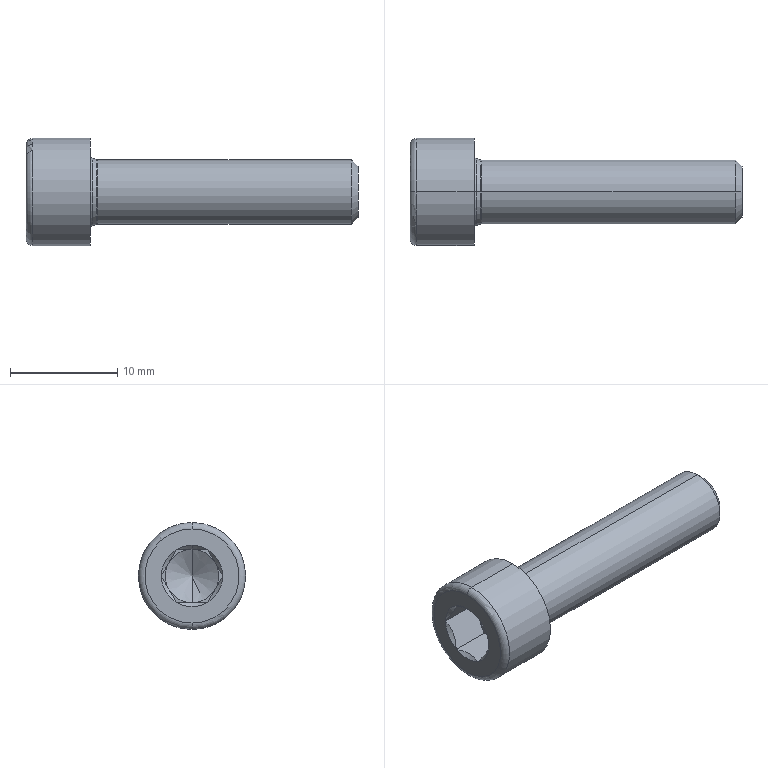Part | STEP file | 1 solid | 38 faces | box 31 x 10 x 10 mm | volume 1084 mm3 | plane 15 | cone 13 | torus 6 | cylinder 4 | commonest cylinder face diameters 6 x2 10 x2
STEP:
#1=CARTESIAN_POINT('',(-0.8566,0.,0.));
#2=VERTEX_POINT('',#1);
#3=CARTESIAN_POINT('',(-2.3,0.,2.5));
#4=VERTEX_POINT('',#3);
#5=CARTESIAN_POINT('',(-2.3,0.,2.5));
#6=DIRECTION('',(-0.5,0.,0.866));
#7=VECTOR('',#6,1000.);
#8=LINE('',#5,#7);
#9=EDGE_CURVE('',#2,#4,#8,.T.);
#10=ORIENTED_EDGE('',*,*,#9,.F.);
#11=CARTESIAN_POINT('',(-2.3,0.,-2.5));
#12=VERTEX_POINT('',#11);
#13=CARTESIAN_POINT('',(-2.3,0.,-2.5));
#14=DIRECTION('',(-0.5,0.,-0.866));
#15=VECTOR('',#14,1000.);
#16=LINE('',#13,#15);
#17=EDGE_CURVE('',#2,#12,#16,.T.);
#18=ORIENTED_EDGE('',*,*,#17,.T.);
#19=CARTESIAN_POINT('',(-2.3,-2.165,-1.25));
#20=VERTEX_POINT('',#19);
#21=CARTESIAN_POINT('',(-2.3,0.,0.));
#22=DIRECTION('',(-1.,0.,0.));
#23=DIRECTION('',(0.,0.,1.));
#24=AXIS2_PLACEMENT_3D('',#21,#22,#23);
#25=CIRCLE('',#24,2.5);
#26=EDGE_CURVE('',#12,#20,#25,.T.);
#27=ORIENTED_EDGE('',*,*,#26,.T.);
#28=CARTESIAN_POINT('',(-2.3,-2.165,1.25));
#29=VERTEX_POINT('',#28);
#30=CARTESIAN_POINT('',(-2.3,0.,0.));
#31=DIRECTION('',(-1.,0.,0.));
#32=DIRECTION('',(0.,0.,1.));
#33=AXIS2_PLACEMENT_3D('',#30,#31,#32);
#34=CIRCLE('',#33,2.5);
#35=EDGE_CURVE('',#20,#29,#34,.T.);
#36=ORIENTED_EDGE('',*,*,#35,.T.);
#37=CARTESIAN_POINT('',(-2.3,0.,0.));
#38=DIRECTION('',(-1.,0.,0.));
#39=DIRECTION('',(0.,0.,1.));
#40=AXIS2_PLACEMENT_3D('',#37,#38,#39);
#41=CIRCLE('',#40,2.5);
#42=EDGE_CURVE('',#29,#4,#41,.T.);
#43=ORIENTED_EDGE('',*,*,#42,.T.);
#44=EDGE_LOOP('',(#10,#18,#27,#36,#43));
#45=FACE_OUTER_BOUND('',#44,.T.);
#46=CARTESIAN_POINT('',(-2.3,0.,0.));
#47=DIRECTION('',(-1.,0.,0.));
#48=DIRECTION('',(0.,0.,1.));
#49=AXIS2_PLACEMENT_3D('',#46,#47,#48);
#50=CONICAL_SURFACE('',#49,2.5,1.047);
#51=ADVANCED_FACE('',(#45),#50,.F.);
#52=CARTESIAN_POINT('',(25.,0.,2.386));
#53=VERTEX_POINT('',#52);
#54=CARTESIAN_POINT('',(25.,0.,-2.386));
#55=VERTEX_POINT('',#54);
#56=CARTESIAN_POINT('',(25.,0.,0.));
#57=DIRECTION('',(-1.,0.,0.));
#58=DIRECTION('',(0.,0.,1.));
#59=AXIS2_PLACEMENT_3D('',#56,#57,#58);
#60=CIRCLE('',#59,2.386);
#61=EDGE_CURVE('',#53,#55,#60,.T.);
#62=ORIENTED_EDGE('',*,*,#61,.T.);
#63=CARTESIAN_POINT('',(24.386,0.,-3.));
#64=VERTEX_POINT('',#63);
#65=CARTESIAN_POINT('',(25.,0.,-2.386));
#66=DIRECTION('',(-0.7071,0.,-0.7071));
#67=VECTOR('',#66,1000.);
#68=LINE('',#65,#67);
#69=EDGE_CURVE('',#55,#64,#68,.T.);
#70=ORIENTED_EDGE('',*,*,#69,.T.);
#71=CARTESIAN_POINT('',(24.386,0.,3.));
#72=VERTEX_POINT('',#71);
#73=CARTESIAN_POINT('',(24.386,0.,0.));
#74=DIRECTION('',(-1.,0.,0.));
#75=DIRECTION('',(0.,0.,1.));
#76=AXIS2_PLACEMENT_3D('',#73,#74,#75);
#77=CIRCLE('',#76,3.);
#78=EDGE_CURVE('',#72,#64,#77,.T.);
#79=ORIENTED_EDGE('',*,*,#78,.F.);
#80=CARTESIAN_POINT('',(25.,0.,2.386));
#81=DIRECTION('',(-0.7071,0.,0.7071));
#82=VECTOR('',#81,1000.);
#83=LINE('',#80,#82);
#84=EDGE_CURVE('',#53,#72,#83,.T.);
#85=ORIENTED_EDGE('',*,*,#84,.F.);
#86=EDGE_LOOP('',(#62,#70,#79,#85));
#87=FACE_OUTER_BOUND('',#86,.T.);
#88=CARTESIAN_POINT('',(25.,0.,0.));
#89=DIRECTION('',(-1.,0.,0.));
#90=DIRECTION('',(0.,0.,1.));
#91=AXIS2_PLACEMENT_3D('',#88,#89,#90);
#92=CONICAL_SURFACE('',#91,2.386,0.7854);
#93=ADVANCED_FACE('',(#87),#92,.T.);
#94=ORIENTED_EDGE('',*,*,#78,.T.);
#95=CARTESIAN_POINT('',(0.68,0.,-3.));
#96=VERTEX_POINT('',#95);
#97=CARTESIAN_POINT('',(28.,0.,-3.));
#98=DIRECTION('',(-1.,0.,0.));
#99=VECTOR('',#98,1000.);
#100=LINE('',#97,#99);
#101=EDGE_CURVE('',#64,#96,#100,.T.);
#102=ORIENTED_EDGE('',*,*,#101,.T.);
#103=CARTESIAN_POINT('',(0.68,0.,3.));
#104=VERTEX_POINT('',#103);
#105=CARTESIAN_POINT('',(0.68,0.,0.));
#106=DIRECTION('',(-1.,0.,0.));
#107=DIRECTION('',(0.,0.,1.));
#108=AXIS2_PLACEMENT_3D('',#105,#106,#107);
#109=CIRCLE('',#108,3.);
#110=EDGE_CURVE('',#104,#96,#109,.T.);
#111=ORIENTED_EDGE('',*,*,#110,.F.);
#112=CARTESIAN_POINT('',(28.,0.,3.));
#113=DIRECTION('',(-1.,0.,0.));
#114=VECTOR('',#113,1000.);
#115=LINE('',#112,#114);
#116=EDGE_CURVE('',#72,#104,#115,.T.);
#117=ORIENTED_EDGE('',*,*,#116,.F.);
#118=EDGE_LOOP('',(#94,#102,#111,#117));
#119=FACE_OUTER_BOUND('',#118,.T.);
#120=CARTESIAN_POINT('',(28.,0.,0.));
#121=DIRECTION('',(-1.,0.,0.));
#122=DIRECTION('',(0.,0.,1.));
#123=AXIS2_PLACEMENT_3D('',#120,#121,#122);
#124=CYLINDRICAL_SURFACE('',#123,3.);
#125=ADVANCED_FACE('',(#119),#124,.T.);
#126=CARTESIAN_POINT('',(0.5977,0.,-3.014));
#127=VERTEX_POINT('',#126);
#128=CARTESIAN_POINT('',(0.5977,0.,3.014));
#129=VERTEX_POINT('',#128);
#130=CARTESIAN_POINT('',(0.5977,0.,0.));
#131=DIRECTION('',(-1.,0.,0.));
#132=DIRECTION('',(0.,0.,1.));
#133=AXIS2_PLACEMENT_3D('',#130,#131,#132);
#134=CIRCLE('',#133,3.014);
#135=EDGE_CURVE('',#127,#129,#134,.T.);
#136=ORIENTED_EDGE('',*,*,#135,.F.);
#137=CARTESIAN_POINT('',(0.68,0.,-3.25));
#138=DIRECTION('',(0.,1.,0.));
#139=DIRECTION('',(0.,0.,1.));
#140=AXIS2_PLACEMENT_3D('',#137,#138,#139);
#141=CIRCLE('',#140,0.25);
#142=EDGE_CURVE('',#127,#96,#141,.T.);
#143=ORIENTED_EDGE('',*,*,#142,.T.);
#144=CARTESIAN_POINT('',(0.68,0.,0.));
#145=DIRECTION('',(-1.,0.,0.));
#146=DIRECTION('',(0.,0.,1.));
#147=AXIS2_PLACEMENT_3D('',#144,#145,#146);
#148=CIRCLE('',#147,3.);
#149=EDGE_CURVE('',#96,#104,#148,.T.);
#150=ORIENTED_EDGE('',*,*,#149,.T.);
#151=CARTESIAN_POINT('',(0.68,0.,3.25));
#152=DIRECTION('',(0.,-1.,0.));
#153=DIRECTION('',(0.,0.,-1.));
#154=AXIS2_PLACEMENT_3D('',#151,#152,#153);
#155=CIRCLE('',#154,0.25);
#156=EDGE_CURVE('',#129,#104,#155,.T.);
#157=ORIENTED_EDGE('',*,*,#156,.F.);
#158=EDGE_LOOP('',(#136,#143,#150,#157));
#159=FACE_OUTER_BOUND('',#158,.T.);
#160=CARTESIAN_POINT('',(0.68,0.,0.));
#161=DIRECTION('',(-1.,0.,0.));
#162=DIRECTION('',(0.,0.,1.));
#163=AXIS2_PLACEMENT_3D('',#160,#161,#162);
#164=TOROIDAL_SURFACE('',#163,3.25,0.25);
#165=ADVANCED_FACE('',(#159),#164,.F.);
#166=CARTESIAN_POINT('',(0.5977,0.,0.));
#167=DIRECTION('',(-1.,0.,0.));
#168=DIRECTION('',(0.,0.,1.));
#169=AXIS2_PLACEMENT_3D('',#166,#167,#168);
#170=CIRCLE('',#169,3.014);
#171=EDGE_CURVE('',#129,#127,#170,.T.);
#172=ORIENTED_EDGE('',*,*,#171,.T.);
#173=CARTESIAN_POINT('',(0.1677,0.,-3.164));
#174=VERTEX_POINT('',#173);
#175=CARTESIAN_POINT('',(0.5977,0.,-3.014));
#176=DIRECTION('',(-0.9442,0.,-0.3294));
#177=VECTOR('',#176,1000.);
#178=LINE('',#175,#177);
#179=EDGE_CURVE('',#127,#174,#178,.T.);
#180=ORIENTED_EDGE('',*,*,#179,.T.);
#181=CARTESIAN_POINT('',(0.1677,0.,3.164));
#182=VERTEX_POINT('',#181);
#183=CARTESIAN_POINT('',(0.1677,0.,0.));
#184=DIRECTION('',(-1.,0.,0.));
#185=DIRECTION('',(0.,0.,1.));
#186=AXIS2_PLACEMENT_3D('',#183,#184,#185);
#187=CIRCLE('',#186,3.164);
#188=EDGE_CURVE('',#182,#174,#187,.T.);
#189=ORIENTED_EDGE('',*,*,#188,.F.);
#190=CARTESIAN_POINT('',(0.5977,0.,3.014));
#191=DIRECTION('',(-0.9442,0.,0.3294));
#192=VECTOR('',#191,1000.);
#193=LINE('',#190,#192);
#194=EDGE_CURVE('',#129,#182,#193,.T.);
#195=ORIENTED_EDGE('',*,*,#194,.F.);
#196=EDGE_LOOP('',(#172,#180,#189,#195));
#197=FACE_OUTER_BOUND('',#196,.T.);
#198=CARTESIAN_POINT('',(0.5977,0.,0.));
#199=DIRECTION('',(-1.,0.,0.));
#200=DIRECTION('',(0.,0.,1.));
#201=AXIS2_PLACEMENT_3D('',#198,#199,#200);
#202=CONICAL_SURFACE('',#201,3.014,0.3356);
#203=ADVANCED_FACE('',(#197),#202,.T.);
#204=CARTESIAN_POINT('',(0.,0.,-3.4));
#205=VERTEX_POINT('',#204);
#206=CARTESIAN_POINT('',(0.,0.,3.4));
#207=VERTEX_POINT('',#206);
#208=CARTESIAN_POINT('',(0.,0.,0.));
#209=DIRECTION('',(-1.,0.,0.));
#210=DIRECTION('',(0.,0.,1.));
#211=AXIS2_PLACEMENT_3D('',#208,#209,#210);
#212=CIRCLE('',#211,3.4);
#213=EDGE_CURVE('',#205,#207,#212,.T.);
#214=ORIENTED_EDGE('',*,*,#213,.F.);
#215=CARTESIAN_POINT('',(0.25,0.,-3.4));
#216=DIRECTION('',(0.,1.,0.));
#217=DIRECTION('',(0.,0.,1.));
#218=AXIS2_PLACEMENT_3D('',#215,#216,#217);
#219=CIRCLE('',#218,0.25);
#220=EDGE_CURVE('',#205,#174,#219,.T.);
#221=ORIENTED_EDGE('',*,*,#220,.T.);
#222=CARTESIAN_POINT('',(0.1677,0.,0.));
#223=DIRECTION('',(-1.,0.,0.));
#224=DIRECTION('',(0.,0.,1.));
#225=AXIS2_PLACEMENT_3D('',#222,#223,#224);
#226=CIRCLE('',#225,3.164);
#227=EDGE_CURVE('',#174,#182,#226,.T.);
#228=ORIENTED_EDGE('',*,*,#227,.T.);
#229=CARTESIAN_POINT('',(0.25,0.,3.4));
#230=DIRECTION('',(0.,-1.,0.));
#231=DIRECTION('',(0.,0.,-1.));
#232=AXIS2_PLACEMENT_3D('',#229,#230,#231);
#233=CIRCLE('',#232,0.25);
#234=EDGE_CURVE('',#207,#182,#233,.T.);
#235=ORIENTED_EDGE('',*,*,#234,.F.);
#236=EDGE_LOOP('',(#214,#221,#228,#235));
#237=FACE_OUTER_BOUND('',#236,.T.);
#238=CARTESIAN_POINT('',(0.25,0.,0.));
#239=DIRECTION('',(-1.,0.,0.));
#240=DIRECTION('',(0.,0.,1.));
#241=AXIS2_PLACEMENT_3D('',#238,#239,#240);
#242=TOROIDAL_SURFACE('',#241,3.4,0.25);
#243=ADVANCED_FACE('',(#237),#242,.F.);
#244=CARTESIAN_POINT('',(0.,0.,5.));
#245=VERTEX_POINT('',#244);
#246=CARTESIAN_POINT('',(0.,0.,-5.));
#247=VERTEX_POINT('',#246);
#248=CARTESIAN_POINT('',(0.,0.,0.));
#249=DIRECTION('',(-1.,0.,0.));
#250=DIRECTION('',(0.,0.,1.));
#251=AXIS2_PLACEMENT_3D('',#248,#249,#250);
#252=CIRCLE('',#251,5.);
#253=EDGE_CURVE('',#245,#247,#252,.T.);
#254=ORIENTED_EDGE('',*,*,#253,.T.);
#255=CARTESIAN_POINT('',(-5.4,0.,-5.));
#256=VERTEX_POINT('',#255);
#257=CARTESIAN_POINT('',(28.,0.,-5.));
#258=DIRECTION('',(-1.,0.,0.));
#259=VECTOR('',#258,1000.);
#260=LINE('',#257,#259);
#261=EDGE_CURVE('',#247,#256,#260,.T.);
#262=ORIENTED_EDGE('',*,*,#261,.T.);
#263=CARTESIAN_POINT('',(-5.4,0.,5.));
#264=VERTEX_POINT('',#263);
#265=CARTESIAN_POINT('',(-5.4,0.,0.));
#266=DIRECTION('',(-1.,0.,0.));
#267=DIRECTION('',(0.,0.,1.));
#268=AXIS2_PLACEMENT_3D('',#265,#266,#267);
#269=CIRCLE('',#268,5.);
#270=EDGE_CURVE('',#264,#256,#269,.T.);
#271=ORIENTED_EDGE('',*,*,#270,.F.);
#272=CARTESIAN_POINT('',(28.,0.,5.));
#273=DIRECTION('',(-1.,0.,0.));
#274=VECTOR('',#273,1000.);
#275=LINE('',#272,#274);
#276=EDGE_CURVE('',#245,#264,#275,.T.);
#277=ORIENTED_EDGE('',*,*,#276,.F.);
#278=EDGE_LOOP('',(#254,#262,#271,#277));
#279=FACE_OUTER_BOUND('',#278,.T.);
#280=CARTESIAN_POINT('',(28.,0.,0.));
#281=DIRECTION('',(-1.,0.,0.));
#282=DIRECTION('',(0.,0.,1.));
#283=AXIS2_PLACEMENT_3D('',#280,#281,#282);
#284=CYLINDRICAL_SURFACE('',#283,5.);
#285=ADVANCED_FACE('',(#279),#284,.T.);
#286=ORIENTED_EDGE('',*,*,#270,.T.);
#287=CARTESIAN_POINT('',(-6.,0.,-4.4));
#288=VERTEX_POINT('',#287);
#289=CARTESIAN_POINT('',(-5.4,0.,-4.4));
#290=DIRECTION('',(0.,1.,0.));
#291=DIRECTION('',(0.,0.,1.));
#292=AXIS2_PLACEMENT_3D('',#289,#290,#291);
#293=CIRCLE('',#292,0.6);
#294=EDGE_CURVE('',#256,#288,#293,.T.);
#295=ORIENTED_EDGE('',*,*,#294,.T.);
#296=CARTESIAN_POINT('',(-6.,0.,4.4));
#297=VERTEX_POINT('',#296);
#298=CARTESIAN_POINT('',(-6.,0.,0.));
#299=DIRECTION('',(-1.,0.,0.));
#300=DIRECTION('',(0.,0.,1.));
#301=AXIS2_PLACEMENT_3D('',#298,#299,#300);
#302=CIRCLE('',#301,4.4);
#303=EDGE_CURVE('',#297,#288,#302,.T.);
#304=ORIENTED_EDGE('',*,*,#303,.F.);
#305=CARTESIAN_POINT('',(-5.4,0.,4.4));
#306=DIRECTION('',(0.,-1.,0.));
#307=DIRECTION('',(0.,0.,-1.));
#308=AXIS2_PLACEMENT_3D('',#305,#306,#307);
#309=CIRCLE('',#308,0.6);
#310=EDGE_CURVE('',#264,#297,#309,.T.);
#311=ORIENTED_EDGE('',*,*,#310,.F.);
#312=EDGE_LOOP('',(#286,#295,#304,#311));
#313=FACE_OUTER_BOUND('',#312,.T.);
#314=CARTESIAN_POINT('',(-5.4,0.,0.));
#315=DIRECTION('',(-1.,0.,0.));
#316=DIRECTION('',(0.,0.,1.));
#317=AXIS2_PLACEMENT_3D('',#314,#315,#316);
#318=TOROIDAL_SURFACE('',#317,4.4,0.6);
#319=ADVANCED_FACE('',(#313),#318,.T.);
#320=CARTESIAN_POINT('',(-6.,1.389,2.5));
#321=VERTEX_POINT('',#320);
#322=CARTESIAN_POINT('',(-5.64,0.,2.5));
#323=VERTEX_POINT('',#322);
#324=CARTESIAN_POINT('',(-6.,1.389,2.5));
#325=CARTESIAN_POINT('',(-5.895,1.173,2.5));
#326=CARTESIAN_POINT('',(-5.804,0.9463,2.5));
#327=CARTESIAN_POINT('',(-5.676,0.481,2.5));
#328=CARTESIAN_POINT('',(-5.64,0.2436,2.5));
#329=CARTESIAN_POINT('',(-5.64,0.,2.5));
#330=B_SPLINE_CURVE_WITH_KNOTS('',3,(#324,#325,#326,#327,#328,#329),.UNSPECIFIED.,.F.,.F.,(4,2,4),(0.001597,0.002315,0.003033),.UNSPECIFIED.);
#331=EDGE_CURVE('',#321,#323,#330,.T.);
#332=ORIENTED_EDGE('',*,*,#331,.T.);
#333=CARTESIAN_POINT('',(-6.,0.,2.86));
#334=VERTEX_POINT('',#333);
#335=CARTESIAN_POINT('',(-6.,0.,2.86));
#336=DIRECTION('',(-0.7071,0.,0.7071));
#337=VECTOR('',#336,1000.);
#338=LINE('',#335,#337);
#339=EDGE_CURVE('',#323,#334,#338,.T.);
#340=ORIENTED_EDGE('',*,*,#339,.T.);
#341=CARTESIAN_POINT('',(-6.,0.,0.));
#342=DIRECTION('',(-1.,0.,0.));
#343=DIRECTION('',(0.,0.,1.));
#344=AXIS2_PLACEMENT_3D('',#341,#342,#343);
#345=CIRCLE('',#344,2.86);
#346=EDGE_CURVE('',#334,#321,#345,.T.);
#347=ORIENTED_EDGE('',*,*,#346,.T.);
#348=EDGE_LOOP('',(#332,#340,#347));
#349=FACE_OUTER_BOUND('',#348,.T.);
#350=CARTESIAN_POINT('',(-6.,0.,0.));
#351=DIRECTION('',(-1.,0.,0.));
#352=DIRECTION('',(0.,0.,1.));
#353=AXIS2_PLACEMENT_3D('',#350,#351,#352);
#354=CONICAL_SURFACE('',#353,2.86,0.7854);
#355=ADVANCED_FACE('',(#349),#354,.F.);
#356=CARTESIAN_POINT('',(-6.,1.471,2.453));
#357=VERTEX_POINT('',#356);
#358=CARTESIAN_POINT('',(-6.,2.86,0.047));
#359=VERTEX_POINT('',#358);
#360=CARTESIAN_POINT('',(-6.,0.,0.));
#361=DIRECTION('',(-1.,0.,0.));
#362=DIRECTION('',(0.,0.,1.));
#363=AXIS2_PLACEMENT_3D('',#360,#361,#362);
#364=CIRCLE('',#363,2.86);
#365=EDGE_CURVE('',#357,#359,#364,.T.);
#366=ORIENTED_EDGE('',*,*,#365,.T.);
#367=CARTESIAN_POINT('',(-6.,2.86,0.047));
#368=CARTESIAN_POINT('',(-5.894,2.751,0.2356));
#369=CARTESIAN_POINT('',(-5.805,2.639,0.4284));
#370=CARTESIAN_POINT('',(-5.709,2.467,0.7273));
#371=CARTESIAN_POINT('',(-5.684,2.408,0.8286));
#372=CARTESIAN_POINT('',(-5.65,2.289,1.035));
#373=CARTESIAN_POINT('',(-5.64,2.228,1.141));
#374=CARTESIAN_POINT('',(-5.64,2.046,1.456));
#375=CARTESIAN_POINT('',(-5.675,1.927,1.661));
#376=CARTESIAN_POINT('',(-5.803,1.693,2.068));
#377=CARTESIAN_POINT('',(-5.894,1.58,2.263));
#378=CARTESIAN_POINT('',(-6.,1.471,2.453));
#379=B_SPLINE_CURVE_WITH_KNOTS('',3,(#367,#368,#369,#370,#371,#372,#373,#374,#375,#376,#377,#378),.UNSPECIFIED.,.F.,.F.,(4,2,2,2,2,4),(0.000000451,0.0007165,0.001075,0.001433,0.002149,0.002865),.UNSPECIFIED.);
#380=EDGE_CURVE('',#359,#357,#379,.T.);
#381=ORIENTED_EDGE('',*,*,#380,.T.);
#382=EDGE_LOOP('',(#366,#381));
#383=FACE_OUTER_BOUND('',#382,.T.);
#384=CARTESIAN_POINT('',(-6.,0.,0.));
#385=DIRECTION('',(-1.,0.,0.));
#386=DIRECTION('',(0.,0.,1.));
#387=AXIS2_PLACEMENT_3D('',#384,#385,#386);
#388=CONICAL_SURFACE('',#387,2.86,0.7854);
#389=ADVANCED_FACE('',(#383),#388,.F.);
#390=CARTESIAN_POINT('',(-6.,2.86,-0.047));
#391=VERTEX_POINT('',#390);
#392=CARTESIAN_POINT('',(-6.,1.471,-2.453));
#393=VERTEX_POINT('',#392);
#394=CARTESIAN_POINT('',(-6.,0.,0.));
#395=DIRECTION('',(-1.,0.,0.));
#396=DIRECTION('',(0.,0.,1.));
#397=AXIS2_PLACEMENT_3D('',#394,#395,#396);
#398=CIRCLE('',#397,2.86);
#399=EDGE_CURVE('',#391,#393,#398,.T.);
#400=ORIENTED_EDGE('',*,*,#399,.T.);
#401=CARTESIAN_POINT('',(-6.,1.471,-2.453));
#402=CARTESIAN_POINT('',(-5.894,1.579,-2.264));
#403=CARTESIAN_POINT('',(-5.805,1.691,-2.072));
#404=CARTESIAN_POINT('',(-5.709,1.863,-1.773));
#405=CARTESIAN_POINT('',(-5.684,1.922,-1.671));
#406=CARTESIAN_POINT('',(-5.65,2.041,-1.465));
#407=CARTESIAN_POINT('',(-5.64,2.102,-1.359));
#408=CARTESIAN_POINT('',(-5.64,2.284,-1.044));
#409=CARTESIAN_POINT('',(-5.675,2.403,-0.8385));
#410=CARTESIAN_POINT('',(-5.803,2.637,-0.4324));
#411=CARTESIAN_POINT('',(-5.894,2.75,-0.2366));
#412=CARTESIAN_POINT('',(-6.,2.86,-0.047));
#413=B_SPLINE_CURVE_WITH_KNOTS('',3,(#401,#402,#403,#404,#405,#406,#407,#408,#409,#410,#411,#412),.UNSPECIFIED.,.F.,.F.,(4,2,2,2,2,4),(0.000000451,0.0007165,0.001075,0.001433,0.002149,0.002865),.UNSPECIFIED.);
#414=EDGE_CURVE('',#393,#391,#413,.T.);
#415=ORIENTED_EDGE('',*,*,#414,.T.);
#416=EDGE_LOOP('',(#400,#415));
#417=FACE_OUTER_BOUND('',#416,.T.);
#418=CARTESIAN_POINT('',(-6.,0.,0.));
#419=DIRECTION('',(-1.,0.,0.));
#420=DIRECTION('',(0.,0.,1.));
#421=AXIS2_PLACEMENT_3D('',#418,#419,#420);
#422=CONICAL_SURFACE('',#421,2.86,0.7854);
#423=ADVANCED_FACE('',(#417),#422,.F.);
#424=CARTESIAN_POINT('',(-6.,1.389,-2.5));
#425=VERTEX_POINT('',#424);
#426=CARTESIAN_POINT('',(-6.,-1.389,-2.5));
#427=VERTEX_POINT('',#426);
#428=CARTESIAN_POINT('',(-6.,0.,0.));
#429=DIRECTION('',(-1.,0.,0.));
#430=DIRECTION('',(0.,0.,1.));
#431=AXIS2_PLACEMENT_3D('',#428,#429,#430);
#432=CIRCLE('',#431,2.86);
#433=EDGE_CURVE('',#425,#427,#432,.T.);
#434=ORIENTED_EDGE('',*,*,#433,.T.);
#435=CARTESIAN_POINT('',(-6.,-1.389,-2.5));
#436=CARTESIAN_POINT('',(-5.895,-1.173,-2.5));
#437=CARTESIAN_POINT('',(-5.804,-0.9455,-2.5));
#438=CARTESIAN_POINT('',(-5.676,-0.482,-2.5));
#439=CARTESIAN_POINT('',(-5.64,-0.2429,-2.5));
#440=CARTESIAN_POINT('',(-5.64,0.2441,-2.5));
#441=CARTESIAN_POINT('',(-5.676,0.4814,-2.5));
#442=CARTESIAN_POINT('',(-5.804,0.9465,-2.5));
#443=CARTESIAN_POINT('',(-5.895,1.173,-2.5));
#444=CARTESIAN_POINT('',(-6.,1.389,-2.5));
#445=B_SPLINE_CURVE_WITH_KNOTS('',3,(#435,#436,#437,#438,#439,#440,#441,#442,#443,#444),.UNSPECIFIED.,.F.,.F.,(4,2,2,2,4),(0.001921,0.002639,0.003357,0.004076,0.004794),.UNSPECIFIED.);
#446=EDGE_CURVE('',#427,#425,#445,.T.);
#447=ORIENTED_EDGE('',*,*,#446,.T.);
#448=EDGE_LOOP('',(#434,#447));
#449=FACE_OUTER_BOUND('',#448,.T.);
#450=CARTESIAN_POINT('',(-6.,0.,0.));
#451=DIRECTION('',(-1.,0.,0.));
#452=DIRECTION('',(0.,0.,1.));
#453=AXIS2_PLACEMENT_3D('',#450,#451,#452);
#454=CONICAL_SURFACE('',#453,2.86,0.7854);
#455=ADVANCED_FACE('',(#449),#454,.F.);
#456=CARTESIAN_POINT('',(-6.,-1.471,-2.453));
#457=VERTEX_POINT('',#456);
#458=CARTESIAN_POINT('',(-6.,-2.86,-0.047));
#459=VERTEX_POINT('',#458);
#460=CARTESIAN_POINT('',(-6.,0.,0.));
#461=DIRECTION('',(-1.,0.,0.));
#462=DIRECTION('',(0.,0.,1.));
#463=AXIS2_PLACEMENT_3D('',#460,#461,#462);
#464=CIRCLE('',#463,2.86);
#465=EDGE_CURVE('',#457,#459,#464,.T.);
#466=ORIENTED_EDGE('',*,*,#465,.T.);
#467=CARTESIAN_POINT('',(-6.,-2.86,-0.047));
#468=CARTESIAN_POINT('',(-5.894,-2.751,-0.2356));
#469=CARTESIAN_POINT('',(-5.805,-2.639,-0.4284));
#470=CARTESIAN_POINT('',(-5.709,-2.467,-0.7273));
#471=CARTESIAN_POINT('',(-5.684,-2.408,-0.8286));
#472=CARTESIAN_POINT('',(-5.65,-2.289,-1.035));
#473=CARTESIAN_POINT('',(-5.64,-2.228,-1.141));
#474=CARTESIAN_POINT('',(-5.64,-2.046,-1.456));
#475=CARTESIAN_POINT('',(-5.675,-1.927,-1.661));
#476=CARTESIAN_POINT('',(-5.803,-1.693,-2.068));
#477=CARTESIAN_POINT('',(-5.894,-1.58,-2.263));
#478=CARTESIAN_POINT('',(-6.,-1.471,-2.453));
#479=B_SPLINE_CURVE_WITH_KNOTS('',3,(#467,#468,#469,#470,#471,#472,#473,#474,#475,#476,#477,#478),.UNSPECIFIED.,.F.,.F.,(4,2,2,2,2,4),(0.000000451,0.0007165,0.001075,0.001433,0.002149,0.002865),.UNSPECIFIED.);
#480=EDGE_CURVE('',#459,#457,#479,.T.);
#481=ORIENTED_EDGE('',*,*,#480,.T.);
#482=EDGE_LOOP('',(#466,#481));
#483=FACE_OUTER_BOUND('',#482,.T.);
#484=CARTESIAN_POINT('',(-6.,0.,0.));
#485=DIRECTION('',(-1.,0.,0.));
#486=DIRECTION('',(0.,0.,1.));
#487=AXIS2_PLACEMENT_3D('',#484,#485,#486);
#488=CONICAL_SURFACE('',#487,2.86,0.7854);
#489=ADVANCED_FACE('',(#483),#488,.F.);
#490=CARTESIAN_POINT('',(-6.,-2.86,0.047));
#491=VERTEX_POINT('',#490);
#492=CARTESIAN_POINT('',(-6.,-1.471,2.453));
#493=VERTEX_POINT('',#492);
#494=CARTESIAN_POINT('',(-6.,0.,0.));
#495=DIRECTION('',(-1.,0.,0.));
#496=DIRECTION('',(0.,0.,1.));
#497=AXIS2_PLACEMENT_3D('',#494,#495,#496);
#498=CIRCLE('',#497,2.86);
#499=EDGE_CURVE('',#491,#493,#498,.T.);
#500=ORIENTED_EDGE('',*,*,#499,.T.);
#501=CARTESIAN_POINT('',(-6.,-1.471,2.453));
#502=CARTESIAN_POINT('',(-5.894,-1.579,2.264));
#503=CARTESIAN_POINT('',(-5.805,-1.691,2.072));
#504=CARTESIAN_POINT('',(-5.709,-1.863,1.773));
#505=CARTESIAN_POINT('',(-5.684,-1.922,1.671));
#506=CARTESIAN_POINT('',(-5.65,-2.041,1.465));
#507=CARTESIAN_POINT('',(-5.64,-2.102,1.359));
#508=CARTESIAN_POINT('',(-5.64,-2.284,1.044));
#509=CARTESIAN_POINT('',(-5.675,-2.403,0.8385));
#510=CARTESIAN_POINT('',(-5.803,-2.637,0.4324));
#511=CARTESIAN_POINT('',(-5.894,-2.75,0.2366));
#512=CARTESIAN_POINT('',(-6.,-2.86,0.047));
#513=B_SPLINE_CURVE_WITH_KNOTS('',3,(#501,#502,#503,#504,#505,#506,#507,#508,#509,#510,#511,#512),.UNSPECIFIED.,.F.,.F.,(4,2,2,2,2,4),(0.000000451,0.0007165,0.001075,0.001433,0.002149,0.002865),.UNSPECIFIED.);
#514=EDGE_CURVE('',#493,#491,#513,.T.);
#515=ORIENTED_EDGE('',*,*,#514,.T.);
#516=EDGE_LOOP('',(#500,#515));
#517=FACE_OUTER_BOUND('',#516,.T.);
#518=CARTESIAN_POINT('',(-6.,0.,0.));
#519=DIRECTION('',(-1.,0.,0.));
#520=DIRECTION('',(0.,0.,1.));
#521=AXIS2_PLACEMENT_3D('',#518,#519,#520);
#522=CONICAL_SURFACE('',#521,2.86,0.7854);
#523=ADVANCED_FACE('',(#517),#522,.F.);
#524=ORIENTED_EDGE('',*,*,#339,.F.);
#525=CARTESIAN_POINT('',(-6.,-1.389,2.5));
#526=VERTEX_POINT('',#525);
#527=CARTESIAN_POINT('',(-5.64,0.,2.5));
#528=CARTESIAN_POINT('',(-5.64,-0.2434,2.5));
#529=CARTESIAN_POINT('',(-5.676,-0.4824,2.5));
#530=CARTESIAN_POINT('',(-5.804,-0.9456,2.5));
#531=CARTESIAN_POINT('',(-5.895,-1.173,2.5));
#532=CARTESIAN_POINT('',(-6.,-1.389,2.5));
#533=B_SPLINE_CURVE_WITH_KNOTS('',3,(#527,#528,#529,#530,#531,#532),.UNSPECIFIED.,.F.,.F.,(4,2,4),(0.003033,0.00375,0.004467),.UNSPECIFIED.);
#534=EDGE_CURVE('',#323,#526,#533,.T.);
#535=ORIENTED_EDGE('',*,*,#534,.T.);
#536=CARTESIAN_POINT('',(-6.,0.,0.));
#537=DIRECTION('',(-1.,0.,0.));
#538=DIRECTION('',(0.,0.,1.));
#539=AXIS2_PLACEMENT_3D('',#536,#537,#538);
#540=CIRCLE('',#539,2.86);
#541=EDGE_CURVE('',#526,#334,#540,.T.);
#542=ORIENTED_EDGE('',*,*,#541,.T.);
#543=EDGE_LOOP('',(#524,#535,#542));
#544=FACE_OUTER_BOUND('',#543,.T.);
#545=CARTESIAN_POINT('',(-6.,0.,0.));
#546=DIRECTION('',(-1.,0.,0.));
#547=DIRECTION('',(0.,0.,1.));
#548=AXIS2_PLACEMENT_3D('',#545,#546,#547);
#549=CONICAL_SURFACE('',#548,2.86,0.7854);
#550=ADVANCED_FACE('',(#544),#549,.F.);
#551=CARTESIAN_POINT('',(-6.,2.887,0.));
#552=VERTEX_POINT('',#551);
#553=CARTESIAN_POINT('',(-6.,2.88,-0.01158));
#554=DIRECTION('',(0.,0.5,0.866));
#555=VECTOR('',#554,1000.);
#556=LINE('',#553,#555);
#557=EDGE_CURVE('',#391,#552,#556,.T.);
#558=ORIENTED_EDGE('',*,*,#557,.T.);
#559=CARTESIAN_POINT('',(-6.,2.88,0.01158));
#560=DIRECTION('',(0.,-0.5,0.866));
#561=VECTOR('',#560,1000.);
#562=LINE('',#559,#561);
#563=EDGE_CURVE('',#552,#359,#562,.T.);
#564=ORIENTED_EDGE('',*,*,#563,.T.);
#565=ORIENTED_EDGE('',*,*,#365,.F.);
#566=CARTESIAN_POINT('',(-6.,1.443,2.5));
#567=VERTEX_POINT('',#566);
#568=CARTESIAN_POINT('',(-6.,2.88,0.01158));
#569=DIRECTION('',(0.,-0.5,0.866));
#570=VECTOR('',#569,1000.);
#571=LINE('',#568,#570);
#572=EDGE_CURVE('',#357,#567,#571,.T.);
#573=ORIENTED_EDGE('',*,*,#572,.T.);
#574=CARTESIAN_POINT('',(-6.,2.86,2.5));
#575=DIRECTION('',(0.,-1.,0.));
#576=VECTOR('',#575,1000.);
#577=LINE('',#574,#576);
#578=EDGE_CURVE('',#567,#321,#577,.T.);
#579=ORIENTED_EDGE('',*,*,#578,.T.);
#580=ORIENTED_EDGE('',*,*,#346,.F.);
#581=ORIENTED_EDGE('',*,*,#541,.F.);
#582=CARTESIAN_POINT('',(-6.,-1.443,2.5));
#583=VERTEX_POINT('',#582);
#584=CARTESIAN_POINT('',(-6.,2.86,2.5));
#585=DIRECTION('',(0.,-1.,0.));
#586=VECTOR('',#585,1000.);
#587=LINE('',#584,#586);
#588=EDGE_CURVE('',#526,#583,#587,.T.);
#589=ORIENTED_EDGE('',*,*,#588,.T.);
#590=CARTESIAN_POINT('',(-6.,-1.45,2.488));
#591=DIRECTION('',(0.,-0.5,-0.866));
#592=VECTOR('',#591,1000.);
#593=LINE('',#590,#592);
#594=EDGE_CURVE('',#583,#493,#593,.T.);
#595=ORIENTED_EDGE('',*,*,#594,.T.);
#596=ORIENTED_EDGE('',*,*,#499,.F.);
#597=CARTESIAN_POINT('',(-6.,-2.887,0.));
#598=VERTEX_POINT('',#597);
#599=CARTESIAN_POINT('',(-6.,-1.45,2.488));
#600=DIRECTION('',(0.,-0.5,-0.866));
#601=VECTOR('',#600,1000.);
#602=LINE('',#599,#601);
#603=EDGE_CURVE('',#491,#598,#602,.T.);
#604=ORIENTED_EDGE('',*,*,#603,.T.);
#605=CARTESIAN_POINT('',(-6.,-1.45,-2.488));
#606=DIRECTION('',(0.,0.5,-0.866));
#607=VECTOR('',#606,1000.);
#608=LINE('',#605,#607);
#609=EDGE_CURVE('',#598,#459,#608,.T.);
#610=ORIENTED_EDGE('',*,*,#609,.T.);
#611=ORIENTED_EDGE('',*,*,#465,.F.);
#612=CARTESIAN_POINT('',(-6.,-1.443,-2.5));
#613=VERTEX_POINT('',#612);
#614=CARTESIAN_POINT('',(-6.,-1.45,-2.488));
#615=DIRECTION('',(0.,0.5,-0.866));
#616=VECTOR('',#615,1000.);
#617=LINE('',#614,#616);
#618=EDGE_CURVE('',#457,#613,#617,.T.);
#619=ORIENTED_EDGE('',*,*,#618,.T.);
#620=CARTESIAN_POINT('',(-6.,2.86,-2.5));
#621=DIRECTION('',(0.,1.,0.));
#622=VECTOR('',#621,1000.);
#623=LINE('',#620,#622);
#624=EDGE_CURVE('',#613,#427,#623,.T.);
#625=ORIENTED_EDGE('',*,*,#624,.T.);
#626=ORIENTED_EDGE('',*,*,#433,.F.);
#627=CARTESIAN_POINT('',(-6.,1.443,-2.5));
#628=VERTEX_POINT('',#627);
#629=CARTESIAN_POINT('',(-6.,2.86,-2.5));
#630=DIRECTION('',(0.,1.,0.));
#631=VECTOR('',#630,1000.);
#632=LINE('',#629,#631);
#633=EDGE_CURVE('',#425,#628,#632,.T.);
#634=ORIENTED_EDGE('',*,*,#633,.T.);
#635=CARTESIAN_POINT('',(-6.,2.88,-0.01158));
#636=DIRECTION('',(0.,0.5,0.866));
#637=VECTOR('',#636,1000.);
#638=LINE('',#635,#637);
#639=EDGE_CURVE('',#628,#393,#638,.T.);
#640=ORIENTED_EDGE('',*,*,#639,.T.);
#641=ORIENTED_EDGE('',*,*,#399,.F.);
#642=EDGE_LOOP('',(#558,#564,#565,#573,#579,#580,#581,#589,#595,#596,#604,#610,#611,#619,#625,#626,#634,#640,#641));
#643=FACE_BOUND('',#642,.T.);
#644=ORIENTED_EDGE('',*,*,#303,.T.);
#645=CARTESIAN_POINT('',(-6.,0.,0.));
#646=DIRECTION('',(-1.,0.,0.));
#647=DIRECTION('',(0.,0.,1.));
#648=AXIS2_PLACEMENT_3D('',#645,#646,#647);
#649=CIRCLE('',#648,4.4);
#650=EDGE_CURVE('',#288,#297,#649,.T.);
#651=ORIENTED_EDGE('',*,*,#650,.T.);
#652=EDGE_LOOP('',(#644,#651));
#653=FACE_OUTER_BOUND('',#652,.T.);
#654=CARTESIAN_POINT('',(-6.,2.86,0.));
#655=DIRECTION('',(1.,0.,0.));
#656=DIRECTION('',(0.,0.,-1.));
#657=AXIS2_PLACEMENT_3D('',#654,#655,#656);
#658=PLANE('',#657);
#659=ADVANCED_FACE('',(#643,#653),#658,.F.);
#660=ORIENTED_EDGE('',*,*,#294,.F.);
#661=CARTESIAN_POINT('',(-5.4,0.,0.));
#662=DIRECTION('',(-1.,0.,0.));
#663=DIRECTION('',(0.,0.,1.));
#664=AXIS2_PLACEMENT_3D('',#661,#662,#663);
#665=CIRCLE('',#664,5.);
#666=EDGE_CURVE('',#256,#264,#665,.T.);
#667=ORIENTED_EDGE('',*,*,#666,.T.);
#668=ORIENTED_EDGE('',*,*,#310,.T.);
#669=ORIENTED_EDGE('',*,*,#650,.F.);
#670=EDGE_LOOP('',(#660,#667,#668,#669));
#671=FACE_OUTER_BOUND('',#670,.T.);
#672=CARTESIAN_POINT('',(-5.4,0.,0.));
#673=DIRECTION('',(-1.,0.,0.));
#674=DIRECTION('',(0.,0.,1.));
#675=AXIS2_PLACEMENT_3D('',#672,#673,#674);
#676=TOROIDAL_SURFACE('',#675,4.4,0.6);
#677=ADVANCED_FACE('',(#671),#676,.T.);
#678=ORIENTED_EDGE('',*,*,#261,.F.);
#679=CARTESIAN_POINT('',(0.,0.,0.));
#680=DIRECTION('',(-1.,0.,0.));
#681=DIRECTION('',(0.,0.,1.));
#682=AXIS2_PLACEMENT_3D('',#679,#680,#681);
#683=CIRCLE('',#682,5.);
#684=EDGE_CURVE('',#247,#245,#683,.T.);
#685=ORIENTED_EDGE('',*,*,#684,.T.);
#686=ORIENTED_EDGE('',*,*,#276,.T.);
#687=ORIENTED_EDGE('',*,*,#666,.F.);
#688=EDGE_LOOP('',(#678,#685,#686,#687));
#689=FACE_OUTER_BOUND('',#688,.T.);
#690=CARTESIAN_POINT('',(28.,0.,0.));
#691=DIRECTION('',(-1.,0.,0.));
#692=DIRECTION('',(0.,0.,1.));
#693=AXIS2_PLACEMENT_3D('',#690,#691,#692);
#694=CYLINDRICAL_SURFACE('',#693,5.);
#695=ADVANCED_FACE('',(#689),#694,.T.);
#696=ORIENTED_EDGE('',*,*,#253,.F.);
#697=ORIENTED_EDGE('',*,*,#684,.F.);
#698=EDGE_LOOP('',(#696,#697));
#699=FACE_OUTER_BOUND('',#698,.T.);
#700=CARTESIAN_POINT('',(0.,0.,0.));
#701=DIRECTION('',(-1.,0.,0.));
#702=DIRECTION('',(0.,0.,1.));
#703=AXIS2_PLACEMENT_3D('',#700,#701,#702);
#704=CIRCLE('',#703,3.4);
#705=EDGE_CURVE('',#207,#205,#704,.T.);
#706=ORIENTED_EDGE('',*,*,#705,.T.);
#707=ORIENTED_EDGE('',*,*,#213,.T.);
#708=EDGE_LOOP('',(#706,#707));
#709=FACE_BOUND('',#708,.T.);
#710=CARTESIAN_POINT('',(0.,5.,0.));
#711=DIRECTION('',(-1.,0.,0.));
#712=DIRECTION('',(0.,0.,1.));
#713=AXIS2_PLACEMENT_3D('',#710,#711,#712);
#714=PLANE('',#713);
#715=ADVANCED_FACE('',(#699,#709),#714,.F.);
#716=ORIENTED_EDGE('',*,*,#220,.F.);
#717=ORIENTED_EDGE('',*,*,#705,.F.);
#718=ORIENTED_EDGE('',*,*,#234,.T.);
#719=ORIENTED_EDGE('',*,*,#188,.T.);
#720=EDGE_LOOP('',(#716,#717,#718,#719));
#721=FACE_OUTER_BOUND('',#720,.T.);
#722=CARTESIAN_POINT('',(0.25,0.,0.));
#723=DIRECTION('',(-1.,0.,0.));
#724=DIRECTION('',(0.,0.,1.));
#725=AXIS2_PLACEMENT_3D('',#722,#723,#724);
#726=TOROIDAL_SURFACE('',#725,3.4,0.25);
#727=ADVANCED_FACE('',(#721),#726,.F.);
#728=ORIENTED_EDGE('',*,*,#179,.F.);
#729=ORIENTED_EDGE('',*,*,#135,.T.);
#730=ORIENTED_EDGE('',*,*,#194,.T.);
#731=ORIENTED_EDGE('',*,*,#227,.F.);
#732=EDGE_LOOP('',(#728,#729,#730,#731));
#733=FACE_OUTER_BOUND('',#732,.T.);
#734=CARTESIAN_POINT('',(0.5977,0.,0.));
#735=DIRECTION('',(-1.,0.,0.));
#736=DIRECTION('',(0.,0.,1.));
#737=AXIS2_PLACEMENT_3D('',#734,#735,#736);
#738=CONICAL_SURFACE('',#737,3.014,0.3356);
#739=ADVANCED_FACE('',(#733),#738,.T.);
#740=ORIENTED_EDGE('',*,*,#142,.F.);
#741=ORIENTED_EDGE('',*,*,#171,.F.);
#742=ORIENTED_EDGE('',*,*,#156,.T.);
#743=ORIENTED_EDGE('',*,*,#110,.T.);
#744=EDGE_LOOP('',(#740,#741,#742,#743));
#745=FACE_OUTER_BOUND('',#744,.T.);
#746=CARTESIAN_POINT('',(0.68,0.,0.));
#747=DIRECTION('',(-1.,0.,0.));
#748=DIRECTION('',(0.,0.,1.));
#749=AXIS2_PLACEMENT_3D('',#746,#747,#748);
#750=TOROIDAL_SURFACE('',#749,3.25,0.25);
#751=ADVANCED_FACE('',(#745),#750,.F.);
#752=ORIENTED_EDGE('',*,*,#101,.F.);
#753=CARTESIAN_POINT('',(24.386,0.,0.));
#754=DIRECTION('',(-1.,0.,0.));
#755=DIRECTION('',(0.,0.,1.));
#756=AXIS2_PLACEMENT_3D('',#753,#754,#755);
#757=CIRCLE('',#756,3.);
#758=EDGE_CURVE('',#64,#72,#757,.T.);
#759=ORIENTED_EDGE('',*,*,#758,.T.);
#760=ORIENTED_EDGE('',*,*,#116,.T.);
#761=ORIENTED_EDGE('',*,*,#149,.F.);
#762=EDGE_LOOP('',(#752,#759,#760,#761));
#763=FACE_OUTER_BOUND('',#762,.T.);
#764=CARTESIAN_POINT('',(28.,0.,0.));
#765=DIRECTION('',(-1.,0.,0.));
#766=DIRECTION('',(0.,0.,1.));
#767=AXIS2_PLACEMENT_3D('',#764,#765,#766);
#768=CYLINDRICAL_SURFACE('',#767,3.);
#769=ADVANCED_FACE('',(#763),#768,.T.);
#770=ORIENTED_EDGE('',*,*,#69,.F.);
#771=CARTESIAN_POINT('',(25.,0.,0.));
#772=DIRECTION('',(-1.,0.,0.));
#773=DIRECTION('',(0.,0.,1.));
#774=AXIS2_PLACEMENT_3D('',#771,#772,#773);
#775=CIRCLE('',#774,2.386);
#776=EDGE_CURVE('',#55,#53,#775,.T.);
#777=ORIENTED_EDGE('',*,*,#776,.T.);
#778=ORIENTED_EDGE('',*,*,#84,.T.);
#779=ORIENTED_EDGE('',*,*,#758,.F.);
#780=EDGE_LOOP('',(#770,#777,#778,#779));
#781=FACE_OUTER_BOUND('',#780,.T.);
#782=CARTESIAN_POINT('',(25.,0.,0.));
#783=DIRECTION('',(-1.,0.,0.));
#784=DIRECTION('',(0.,0.,1.));
#785=AXIS2_PLACEMENT_3D('',#782,#783,#784);
#786=CONICAL_SURFACE('',#785,2.386,0.7854);
#787=ADVANCED_FACE('',(#781),#786,.T.);
#788=ORIENTED_EDGE('',*,*,#61,.F.);
#789=ORIENTED_EDGE('',*,*,#776,.F.);
#790=EDGE_LOOP('',(#788,#789));
#791=FACE_OUTER_BOUND('',#790,.T.);
#792=CARTESIAN_POINT('',(25.,2.386,0.));
#793=DIRECTION('',(-1.,0.,0.));
#794=DIRECTION('',(0.,0.,1.));
#795=AXIS2_PLACEMENT_3D('',#792,#793,#794);
#796=PLANE('',#795);
#797=ADVANCED_FACE('',(#791),#796,.F.);
#798=CARTESIAN_POINT('',(-2.3,-1.443,-2.5));
#799=VERTEX_POINT('',#798);
#800=CARTESIAN_POINT('',(-2.3,-1.443,-2.5));
#801=DIRECTION('',(0.,1.,0.));
#802=VECTOR('',#801,1000.);
#803=LINE('',#800,#802);
#804=EDGE_CURVE('',#799,#12,#803,.T.);
#805=ORIENTED_EDGE('',*,*,#804,.F.);
#806=CARTESIAN_POINT('',(-2.3,-2.887,0.));
#807=DIRECTION('',(0.,0.5,-0.866));
#808=VECTOR('',#807,1000.);
#809=LINE('',#806,#808);
#810=EDGE_CURVE('',#20,#799,#809,.T.);
#811=ORIENTED_EDGE('',*,*,#810,.F.);
#812=ORIENTED_EDGE('',*,*,#26,.F.);
#813=EDGE_LOOP('',(#805,#811,#812));
#814=FACE_OUTER_BOUND('',#813,.T.);
#815=CARTESIAN_POINT('',(-2.3,1.443,2.5));
#816=DIRECTION('',(1.,0.,0.));
#817=DIRECTION('',(0.,0.,-1.));
#818=AXIS2_PLACEMENT_3D('',#815,#816,#817);
#819=PLANE('',#818);
#820=ADVANCED_FACE('',(#814),#819,.F.);
#821=CARTESIAN_POINT('',(-2.3,-2.887,0.));
#822=VERTEX_POINT('',#821);
#823=CARTESIAN_POINT('',(-2.3,-2.887,0.));
#824=DIRECTION('',(0.,0.5,-0.866));
#825=VECTOR('',#824,1000.);
#826=LINE('',#823,#825);
#827=EDGE_CURVE('',#822,#20,#826,.T.);
#828=ORIENTED_EDGE('',*,*,#827,.F.);
#829=CARTESIAN_POINT('',(-2.3,-1.443,2.5));
#830=DIRECTION('',(0.,-0.5,-0.866));
#831=VECTOR('',#830,1000.);
#832=LINE('',#829,#831);
#833=EDGE_CURVE('',#29,#822,#832,.T.);
#834=ORIENTED_EDGE('',*,*,#833,.F.);
#835=ORIENTED_EDGE('',*,*,#35,.F.);
#836=EDGE_LOOP('',(#828,#834,#835));
#837=FACE_OUTER_BOUND('',#836,.T.);
#838=CARTESIAN_POINT('',(-2.3,1.443,2.5));
#839=DIRECTION('',(1.,0.,0.));
#840=DIRECTION('',(0.,0.,-1.));
#841=AXIS2_PLACEMENT_3D('',#838,#839,#840);
#842=PLANE('',#841);
#843=ADVANCED_FACE('',(#837),#842,.F.);
#844=CARTESIAN_POINT('',(-2.3,-1.443,2.5));
#845=VERTEX_POINT('',#844);
#846=CARTESIAN_POINT('',(-2.3,-1.443,2.5));
#847=DIRECTION('',(0.,-0.5,-0.866));
#848=VECTOR('',#847,1000.);
#849=LINE('',#846,#848);
#850=EDGE_CURVE('',#845,#29,#849,.T.);
#851=ORIENTED_EDGE('',*,*,#850,.F.);
#852=CARTESIAN_POINT('',(-2.3,1.443,2.5));
#853=DIRECTION('',(0.,-1.,0.));
#854=VECTOR('',#853,1000.);
#855=LINE('',#852,#854);
#856=EDGE_CURVE('',#4,#845,#855,.T.);
#857=ORIENTED_EDGE('',*,*,#856,.F.);
#858=ORIENTED_EDGE('',*,*,#42,.F.);
#859=EDGE_LOOP('',(#851,#857,#858));
#860=FACE_OUTER_BOUND('',#859,.T.);
#861=CARTESIAN_POINT('',(-2.3,1.443,2.5));
#862=DIRECTION('',(1.,0.,0.));
#863=DIRECTION('',(0.,0.,-1.));
#864=AXIS2_PLACEMENT_3D('',#861,#862,#863);
#865=PLANE('',#864);
#866=ADVANCED_FACE('',(#860),#865,.F.);
#867=CARTESIAN_POINT('',(-2.3,1.443,2.5));
#868=VERTEX_POINT('',#867);
#869=CARTESIAN_POINT('',(-2.3,1.443,2.5));
#870=DIRECTION('',(0.,-1.,0.));
#871=VECTOR('',#870,1000.);
#872=LINE('',#869,#871);
#873=EDGE_CURVE('',#868,#4,#872,.T.);
#874=ORIENTED_EDGE('',*,*,#873,.F.);
#875=CARTESIAN_POINT('',(-2.3,2.165,1.25));
#876=VERTEX_POINT('',#875);
#877=CARTESIAN_POINT('',(-2.3,2.887,0.));
#878=DIRECTION('',(0.,-0.5,0.866));
#879=VECTOR('',#878,1000.);
#880=LINE('',#877,#879);
#881=EDGE_CURVE('',#876,#868,#880,.T.);
#882=ORIENTED_EDGE('',*,*,#881,.F.);
#883=CARTESIAN_POINT('',(-2.3,0.,0.));
#884=DIRECTION('',(-1.,0.,0.));
#885=DIRECTION('',(0.,0.,1.));
#886=AXIS2_PLACEMENT_3D('',#883,#884,#885);
#887=CIRCLE('',#886,2.5);
#888=EDGE_CURVE('',#4,#876,#887,.T.);
#889=ORIENTED_EDGE('',*,*,#888,.F.);
#890=EDGE_LOOP('',(#874,#882,#889));
#891=FACE_OUTER_BOUND('',#890,.T.);
#892=CARTESIAN_POINT('',(-2.3,1.443,2.5));
#893=DIRECTION('',(1.,0.,0.));
#894=DIRECTION('',(0.,0.,-1.));
#895=AXIS2_PLACEMENT_3D('',#892,#893,#894);
#896=PLANE('',#895);
#897=ADVANCED_FACE('',(#891),#896,.F.);
#898=CARTESIAN_POINT('',(-2.3,2.887,0.));
#899=VERTEX_POINT('',#898);
#900=CARTESIAN_POINT('',(-2.3,2.887,0.));
#901=DIRECTION('',(0.,-0.5,0.866));
#902=VECTOR('',#901,1000.);
#903=LINE('',#900,#902);
#904=EDGE_CURVE('',#899,#876,#903,.T.);
#905=ORIENTED_EDGE('',*,*,#904,.F.);
#906=CARTESIAN_POINT('',(-2.3,2.165,-1.25));
#907=VERTEX_POINT('',#906);
#908=CARTESIAN_POINT('',(-2.3,1.443,-2.5));
#909=DIRECTION('',(0.,0.5,0.866));
#910=VECTOR('',#909,1000.);
#911=LINE('',#908,#910);
#912=EDGE_CURVE('',#907,#899,#911,.T.);
#913=ORIENTED_EDGE('',*,*,#912,.F.);
#914=CARTESIAN_POINT('',(-2.3,0.,0.));
#915=DIRECTION('',(-1.,0.,0.));
#916=DIRECTION('',(0.,0.,1.));
#917=AXIS2_PLACEMENT_3D('',#914,#915,#916);
#918=CIRCLE('',#917,2.5);
#919=EDGE_CURVE('',#876,#907,#918,.T.);
#920=ORIENTED_EDGE('',*,*,#919,.F.);
#921=EDGE_LOOP('',(#905,#913,#920));
#922=FACE_OUTER_BOUND('',#921,.T.);
#923=CARTESIAN_POINT('',(-2.3,1.443,2.5));
#924=DIRECTION('',(1.,0.,0.));
#925=DIRECTION('',(0.,0.,-1.));
#926=AXIS2_PLACEMENT_3D('',#923,#924,#925);
#927=PLANE('',#926);
#928=ADVANCED_FACE('',(#922),#927,.F.);
#929=CARTESIAN_POINT('',(-2.3,1.443,-2.5));
#930=VERTEX_POINT('',#929);
#931=CARTESIAN_POINT('',(-2.3,1.443,-2.5));
#932=DIRECTION('',(0.,0.5,0.866));
#933=VECTOR('',#932,1000.);
#934=LINE('',#931,#933);
#935=EDGE_CURVE('',#930,#907,#934,.T.);
#936=ORIENTED_EDGE('',*,*,#935,.F.);
#937=CARTESIAN_POINT('',(-2.3,-1.443,-2.5));
#938=DIRECTION('',(0.,1.,0.));
#939=VECTOR('',#938,1000.);
#940=LINE('',#937,#939);
#941=EDGE_CURVE('',#12,#930,#940,.T.);
#942=ORIENTED_EDGE('',*,*,#941,.F.);
#943=CARTESIAN_POINT('',(-2.3,0.,0.));
#944=DIRECTION('',(-1.,0.,0.));
#945=DIRECTION('',(0.,0.,1.));
#946=AXIS2_PLACEMENT_3D('',#943,#944,#945);
#947=CIRCLE('',#946,2.5);
#948=EDGE_CURVE('',#907,#12,#947,.T.);
#949=ORIENTED_EDGE('',*,*,#948,.F.);
#950=EDGE_LOOP('',(#936,#942,#949));
#951=FACE_OUTER_BOUND('',#950,.T.);
#952=CARTESIAN_POINT('',(-2.3,1.443,2.5));
#953=DIRECTION('',(1.,0.,0.));
#954=DIRECTION('',(0.,0.,-1.));
#955=AXIS2_PLACEMENT_3D('',#952,#953,#954);
#956=PLANE('',#955);
#957=ADVANCED_FACE('',(#951),#956,.F.);
#958=ORIENTED_EDGE('',*,*,#380,.F.);
#959=ORIENTED_EDGE('',*,*,#563,.F.);
#960=CARTESIAN_POINT('',(-8.3,2.887,0.));
#961=DIRECTION('',(1.,0.,0.));
#962=VECTOR('',#961,1000.);
#963=LINE('',#960,#962);
#964=EDGE_CURVE('',#552,#899,#963,.T.);
#965=ORIENTED_EDGE('',*,*,#964,.T.);
#966=ORIENTED_EDGE('',*,*,#904,.T.);
#967=ORIENTED_EDGE('',*,*,#881,.T.);
#968=CARTESIAN_POINT('',(-8.3,1.443,2.5));
#969=DIRECTION('',(1.,0.,0.));
#970=VECTOR('',#969,1000.);
#971=LINE('',#968,#970);
#972=EDGE_CURVE('',#567,#868,#971,.T.);
#973=ORIENTED_EDGE('',*,*,#972,.F.);
#974=ORIENTED_EDGE('',*,*,#572,.F.);
#975=EDGE_LOOP('',(#958,#959,#965,#966,#967,#973,#974));
#976=FACE_OUTER_BOUND('',#975,.T.);
#977=CARTESIAN_POINT('',(-8.3,2.887,0.));
#978=DIRECTION('',(0.,0.866,0.5));
#979=DIRECTION('',(0.,-0.5,0.866));
#980=AXIS2_PLACEMENT_3D('',#977,#978,#979);
#981=PLANE('',#980);
#982=ADVANCED_FACE('',(#976),#981,.F.);
#983=ORIENTED_EDGE('',*,*,#414,.F.);
#984=ORIENTED_EDGE('',*,*,#639,.F.);
#985=CARTESIAN_POINT('',(-8.3,1.443,-2.5));
#986=DIRECTION('',(1.,0.,0.));
#987=VECTOR('',#986,1000.);
#988=LINE('',#985,#987);
#989=EDGE_CURVE('',#628,#930,#988,.T.);
#990=ORIENTED_EDGE('',*,*,#989,.T.);
#991=ORIENTED_EDGE('',*,*,#935,.T.);
#992=ORIENTED_EDGE('',*,*,#912,.T.);
#993=ORIENTED_EDGE('',*,*,#964,.F.);
#994=ORIENTED_EDGE('',*,*,#557,.F.);
#995=EDGE_LOOP('',(#983,#984,#990,#991,#992,#993,#994));
#996=FACE_OUTER_BOUND('',#995,.T.);
#997=CARTESIAN_POINT('',(-8.3,1.443,-2.5));
#998=DIRECTION('',(0.,0.866,-0.5));
#999=DIRECTION('',(0.,0.5,0.866));
#1000=AXIS2_PLACEMENT_3D('',#997,#998,#999);
#1001=PLANE('',#1000);
#1002=ADVANCED_FACE('',(#996),#1001,.F.);
#1003=ORIENTED_EDGE('',*,*,#446,.F.);
#1004=ORIENTED_EDGE('',*,*,#624,.F.);
#1005=CARTESIAN_POINT('',(-8.3,-1.443,-2.5));
#1006=DIRECTION('',(1.,0.,0.));
#1007=VECTOR('',#1006,1000.);
#1008=LINE('',#1005,#1007);
#1009=EDGE_CURVE('',#613,#799,#1008,.T.);
#1010=ORIENTED_EDGE('',*,*,#1009,.T.);
#1011=ORIENTED_EDGE('',*,*,#804,.T.);
#1012=ORIENTED_EDGE('',*,*,#941,.T.);
#1013=ORIENTED_EDGE('',*,*,#989,.F.);
#1014=ORIENTED_EDGE('',*,*,#633,.F.);
#1015=EDGE_LOOP('',(#1003,#1004,#1010,#1011,#1012,#1013,#1014));
#1016=FACE_OUTER_BOUND('',#1015,.T.);
#1017=CARTESIAN_POINT('',(-8.3,-1.443,-2.5));
#1018=DIRECTION('',(0.,0.,-1.));
#1019=DIRECTION('',(-1.,0.,0.));
#1020=AXIS2_PLACEMENT_3D('',#1017,#1018,#1019);
#1021=PLANE('',#1020);
#1022=ADVANCED_FACE('',(#1016),#1021,.F.);
#1023=ORIENTED_EDGE('',*,*,#480,.F.);
#1024=ORIENTED_EDGE('',*,*,#609,.F.);
#1025=CARTESIAN_POINT('',(-8.3,-2.887,0.));
#1026=DIRECTION('',(1.,0.,0.));
#1027=VECTOR('',#1026,1000.);
#1028=LINE('',#1025,#1027);
#1029=EDGE_CURVE('',#598,#822,#1028,.T.);
#1030=ORIENTED_EDGE('',*,*,#1029,.T.);
#1031=ORIENTED_EDGE('',*,*,#827,.T.);
#1032=ORIENTED_EDGE('',*,*,#810,.T.);
#1033=ORIENTED_EDGE('',*,*,#1009,.F.);
#1034=ORIENTED_EDGE('',*,*,#618,.F.);
#1035=EDGE_LOOP('',(#1023,#1024,#1030,#1031,#1032,#1033,#1034));
#1036=FACE_OUTER_BOUND('',#1035,.T.);
#1037=CARTESIAN_POINT('',(-8.3,-2.887,0.));
#1038=DIRECTION('',(0.,-0.866,-0.5));
#1039=DIRECTION('',(0.,0.5,-0.866));
#1040=AXIS2_PLACEMENT_3D('',#1037,#1038,#1039);
#1041=PLANE('',#1040);
#1042=ADVANCED_FACE('',(#1036),#1041,.F.);
#1043=ORIENTED_EDGE('',*,*,#514,.F.);
#1044=ORIENTED_EDGE('',*,*,#594,.F.);
#1045=CARTESIAN_POINT('',(-8.3,-1.443,2.5));
#1046=DIRECTION('',(1.,0.,0.));
#1047=VECTOR('',#1046,1000.);
#1048=LINE('',#1045,#1047);
#1049=EDGE_CURVE('',#583,#845,#1048,.T.);
#1050=ORIENTED_EDGE('',*,*,#1049,.T.);
#1051=ORIENTED_EDGE('',*,*,#850,.T.);
#1052=ORIENTED_EDGE('',*,*,#833,.T.);
#1053=ORIENTED_EDGE('',*,*,#1029,.F.);
#1054=ORIENTED_EDGE('',*,*,#603,.F.);
#1055=EDGE_LOOP('',(#1043,#1044,#1050,#1051,#1052,#1053,#1054));
#1056=FACE_OUTER_BOUND('',#1055,.T.);
#1057=CARTESIAN_POINT('',(-8.3,-1.443,2.5));
#1058=DIRECTION('',(0.,-0.866,0.5));
#1059=DIRECTION('',(0.,-0.5,-0.866));
#1060=AXIS2_PLACEMENT_3D('',#1057,#1058,#1059);
#1061=PLANE('',#1060);
#1062=ADVANCED_FACE('',(#1056),#1061,.F.);
#1063=ORIENTED_EDGE('',*,*,#331,.F.);
#1064=ORIENTED_EDGE('',*,*,#578,.F.);
#1065=ORIENTED_EDGE('',*,*,#972,.T.);
#1066=ORIENTED_EDGE('',*,*,#873,.T.);
#1067=ORIENTED_EDGE('',*,*,#856,.T.);
#1068=ORIENTED_EDGE('',*,*,#1049,.F.);
#1069=ORIENTED_EDGE('',*,*,#588,.F.);
#1070=ORIENTED_EDGE('',*,*,#534,.F.);
#1071=EDGE_LOOP('',(#1063,#1064,#1065,#1066,#1067,#1068,#1069,#1070));
#1072=FACE_OUTER_BOUND('',#1071,.T.);
#1073=CARTESIAN_POINT('',(-8.3,1.443,2.5));
#1074=DIRECTION('',(0.,0.,1.));
#1075=DIRECTION('',(1.,0.,0.));
#1076=AXIS2_PLACEMENT_3D('',#1073,#1074,#1075);
#1077=PLANE('',#1076);
#1078=ADVANCED_FACE('',(#1072),#1077,.F.);
#1079=ORIENTED_EDGE('',*,*,#17,.F.);
#1080=ORIENTED_EDGE('',*,*,#9,.T.);
#1081=ORIENTED_EDGE('',*,*,#888,.T.);
#1082=ORIENTED_EDGE('',*,*,#919,.T.);
#1083=ORIENTED_EDGE('',*,*,#948,.T.);
#1084=EDGE_LOOP('',(#1079,#1080,#1081,#1082,#1083));
#1085=FACE_OUTER_BOUND('',#1084,.T.);
#1086=CARTESIAN_POINT('',(-2.3,0.,0.));
#1087=DIRECTION('',(-1.,0.,0.));
#1088=DIRECTION('',(0.,0.,1.));
#1089=AXIS2_PLACEMENT_3D('',#1086,#1087,#1088);
#1090=CONICAL_SURFACE('',#1089,2.5,1.047);
#1091=ADVANCED_FACE('',(#1085),#1090,.F.);
#1092=CLOSED_SHELL('',(#51,#93,#125,#165,#203,#243,#285,#319,#355,#389,#423,#455,#489,#523,#550,#659,#677,#695,#715,#727,#739,#751,#769,#787,#797,#820,#843,#866,#897,#928,#957,#982,#1002,#1022,#1042,#1062,#1078,#1091));
#1093=MANIFOLD_SOLID_BREP('',#1092);
#1094=CARTESIAN_POINT('',(0.,0.,0.));
#1095=DIRECTION('',(0.,0.,1.));
#1096=DIRECTION('',(1.,0.,0.));
#1097=AXIS2_PLACEMENT_3D('',#1094,#1095,#1096);
#1098=(LENGTH_UNIT()NAMED_UNIT(*)SI_UNIT(.MILLI.,.METRE.));
#1099=UNCERTAINTY_MEASURE_WITH_UNIT(LENGTH_MEASURE(0.00001),#1098,'','');
#1100=(NAMED_UNIT(*)PLANE_ANGLE_UNIT()SI_UNIT($,.RADIAN.));
#1101=(NAMED_UNIT(*)SI_UNIT($,.STERADIAN.)SOLID_ANGLE_UNIT());
#1102=(GEOMETRIC_REPRESENTATION_CONTEXT(3)GLOBAL_UNCERTAINTY_ASSIGNED_CONTEXT((#1099))GLOBAL_UNIT_ASSIGNED_CONTEXT((#1098,#1100,#1101))REPRESENTATION_CONTEXT('',''));
#1103=ADVANCED_BREP_SHAPE_REPRESENTATION('',(#1093,#1097),#1102);